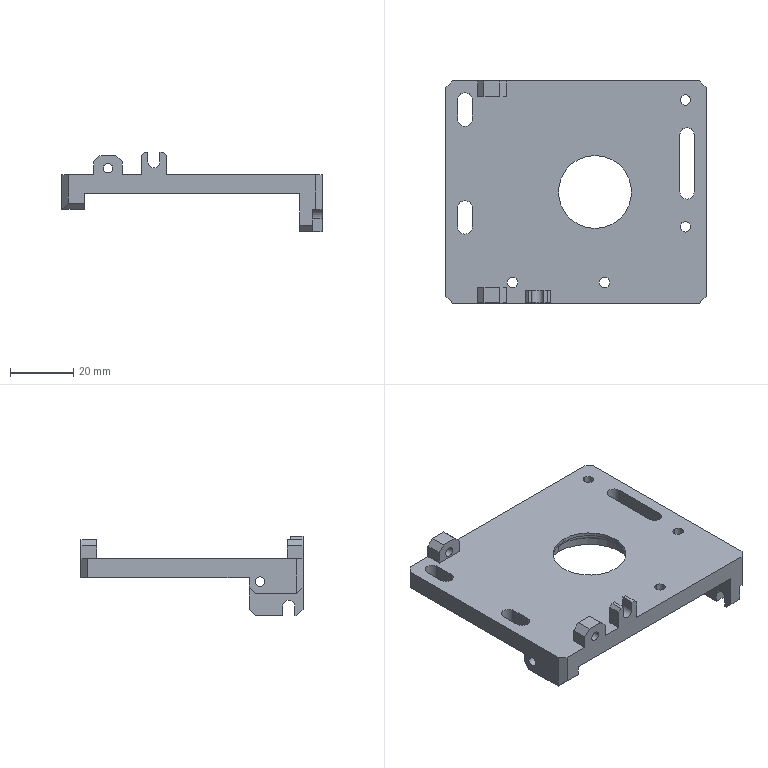NC program | NX | posted with a generic post | part box 82 x 70 x 25 mm
Lines 4669 to 4705 of 8354:
(FLOOR_WALL_1_COPY_COPY , TOOL : D2)
N9300 T08 M6
N9302 G54
N9304 G17 G0 G90 X-20.501 Y30.512 S9500 M3
N9306 G43 Z30. H8
N9308 Z-11.5
N9310 G94 G1 Y33. Z-12.167 F1350.
N9312 Y-33.
N9314 X-21.5
N9316 Y33.
N9318 X-22.5
N9320 Y-33.
N9322 Z-11.667
N9324 G0 Z30.
N9326 X-20.501 Y30.512
N9328 Z-11.667
N9330 G1 Y33. Z-12.333
N9332 Y-33.
N9334 X-21.5
N9336 Y33.
N9338 X-22.5
N9340 Y-33.
N9342 Z-11.833
N9344 G0 Z30.
N9346 X-20.501 Y30.512
N9348 Z-11.833
N9350 G1 Y33. Z-12.5
N9352 Y-33.
N9354 X-21.5
N9356 Y33.
N9358 X-22.5
N9360 Y-33.
N9362 Z-12.
N9364 G0 Z30.
N9366 M5